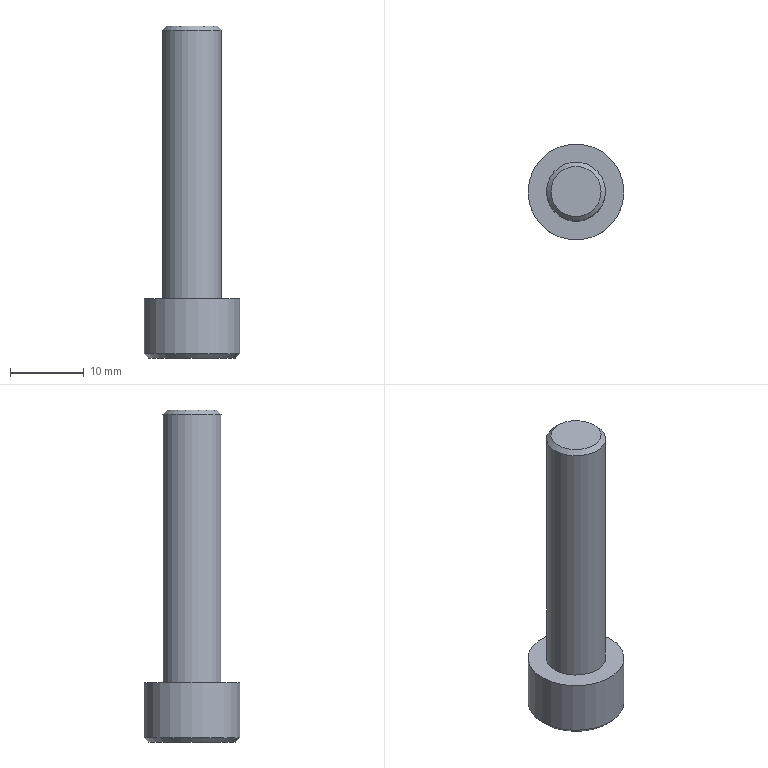Part | STEP file | M8.00-45.00 | 1 solid | 14 faces | box 13 x 13 x 45 mm | volume 2750 mm3 | plane 10 | cylinder 2 | cone 2 | commonest cylinder face diameters 8 x1 13 x1